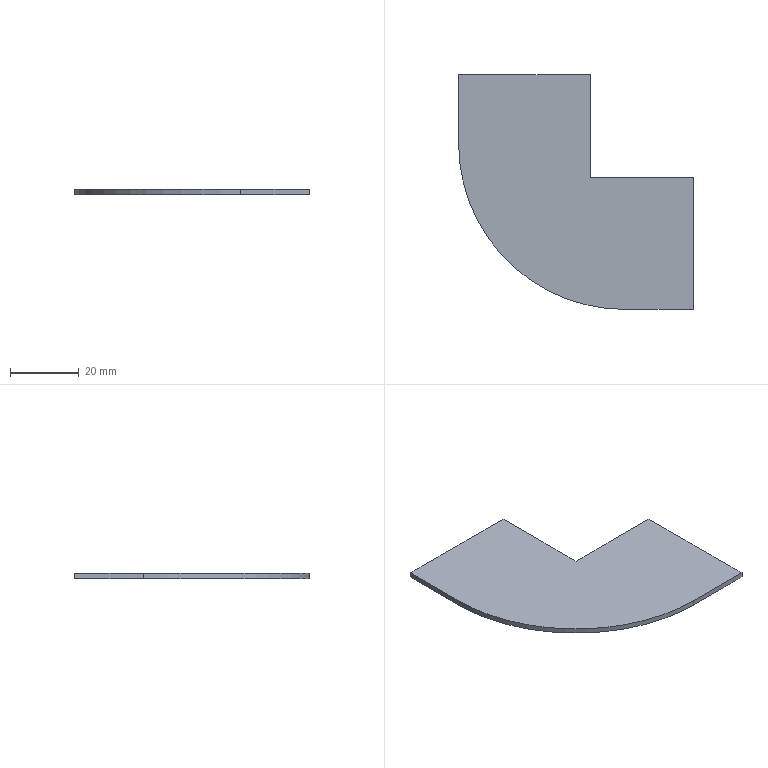Part | SolidWorks | features MirrorStock 1 | 1 solid | 9 faces | box 68.3 x 68.3 x 1.5 mm | volume 4896 mm3 | plane 8 | cylinder 1 | commonest cylinder face diameters 96.6 x1
STEP:
#1=CARTESIAN_POINT('',(9.455,94.386,0.));
#2=VERTEX_POINT('',#1);
#3=CARTESIAN_POINT('',(-28.845,94.386,0.));
#4=VERTEX_POINT('',#3);
#5=CARTESIAN_POINT('',(9.455,94.386,0.));
#6=DIRECTION('',(-1.,0.,0.));
#7=VECTOR('',#6,1000.);
#8=LINE('',#5,#7);
#9=EDGE_CURVE('',#2,#4,#8,.T.);
#10=ORIENTED_EDGE('',*,*,#9,.T.);
#11=CARTESIAN_POINT('',(-28.845,94.386,1.5));
#12=VERTEX_POINT('',#11);
#13=CARTESIAN_POINT('',(-28.845,94.386,1.5));
#14=DIRECTION('',(0.,0.,-1.));
#15=VECTOR('',#14,1000.);
#16=LINE('',#13,#15);
#17=EDGE_CURVE('',#12,#4,#16,.T.);
#18=ORIENTED_EDGE('',*,*,#17,.F.);
#19=CARTESIAN_POINT('',(9.455,94.386,1.5));
#20=VERTEX_POINT('',#19);
#21=CARTESIAN_POINT('',(9.455,94.386,1.5));
#22=DIRECTION('',(-1.,0.,0.));
#23=VECTOR('',#22,1000.);
#24=LINE('',#21,#23);
#25=EDGE_CURVE('',#20,#12,#24,.T.);
#26=ORIENTED_EDGE('',*,*,#25,.F.);
#27=CARTESIAN_POINT('',(9.455,94.386,1.5));
#28=DIRECTION('',(0.,0.,-1.));
#29=VECTOR('',#28,1000.);
#30=LINE('',#27,#29);
#31=EDGE_CURVE('',#20,#2,#30,.T.);
#32=ORIENTED_EDGE('',*,*,#31,.T.);
#33=EDGE_LOOP('',(#10,#18,#26,#32));
#34=FACE_OUTER_BOUND('',#33,.T.);
#35=CARTESIAN_POINT('',(9.455,94.386,1.5));
#36=DIRECTION('',(0.,1.,0.));
#37=DIRECTION('',(0.,0.,-1.));
#38=AXIS2_PLACEMENT_3D('',#35,#36,#37);
#39=PLANE('',#38);
#40=ADVANCED_FACE('',(#34),#39,.T.);
#41=CARTESIAN_POINT('',(9.455,64.386,0.));
#42=VERTEX_POINT('',#41);
#43=CARTESIAN_POINT('',(9.455,64.386,0.));
#44=DIRECTION('',(0.,1.,0.));
#45=VECTOR('',#44,1000.);
#46=LINE('',#43,#45);
#47=EDGE_CURVE('',#42,#2,#46,.T.);
#48=ORIENTED_EDGE('',*,*,#47,.T.);
#49=ORIENTED_EDGE('',*,*,#31,.F.);
#50=CARTESIAN_POINT('',(9.455,64.386,1.5));
#51=VERTEX_POINT('',#50);
#52=CARTESIAN_POINT('',(9.455,64.386,1.5));
#53=DIRECTION('',(0.,1.,0.));
#54=VECTOR('',#53,1000.);
#55=LINE('',#52,#54);
#56=EDGE_CURVE('',#51,#20,#55,.T.);
#57=ORIENTED_EDGE('',*,*,#56,.F.);
#58=CARTESIAN_POINT('',(9.455,64.386,1.5));
#59=DIRECTION('',(0.,0.,-1.));
#60=VECTOR('',#59,1000.);
#61=LINE('',#58,#60);
#62=EDGE_CURVE('',#51,#42,#61,.T.);
#63=ORIENTED_EDGE('',*,*,#62,.T.);
#64=EDGE_LOOP('',(#48,#49,#57,#63));
#65=FACE_OUTER_BOUND('',#64,.T.);
#66=CARTESIAN_POINT('',(9.455,64.386,1.5));
#67=DIRECTION('',(1.,0.,0.));
#68=DIRECTION('',(0.,0.,1.));
#69=AXIS2_PLACEMENT_3D('',#66,#67,#68);
#70=PLANE('',#69);
#71=ADVANCED_FACE('',(#65),#70,.T.);
#72=CARTESIAN_POINT('',(39.455,64.386,0.));
#73=VERTEX_POINT('',#72);
#74=CARTESIAN_POINT('',(39.455,64.386,0.));
#75=DIRECTION('',(-1.,0.,0.));
#76=VECTOR('',#75,1000.);
#77=LINE('',#74,#76);
#78=EDGE_CURVE('',#73,#42,#77,.T.);
#79=ORIENTED_EDGE('',*,*,#78,.T.);
#80=ORIENTED_EDGE('',*,*,#62,.F.);
#81=CARTESIAN_POINT('',(39.455,64.386,1.5));
#82=VERTEX_POINT('',#81);
#83=CARTESIAN_POINT('',(39.455,64.386,1.5));
#84=DIRECTION('',(-1.,0.,0.));
#85=VECTOR('',#84,1000.);
#86=LINE('',#83,#85);
#87=EDGE_CURVE('',#82,#51,#86,.T.);
#88=ORIENTED_EDGE('',*,*,#87,.F.);
#89=CARTESIAN_POINT('',(39.455,64.386,1.5));
#90=DIRECTION('',(0.,0.,-1.));
#91=VECTOR('',#90,1000.);
#92=LINE('',#89,#91);
#93=EDGE_CURVE('',#82,#73,#92,.T.);
#94=ORIENTED_EDGE('',*,*,#93,.T.);
#95=EDGE_LOOP('',(#79,#80,#88,#94));
#96=FACE_OUTER_BOUND('',#95,.T.);
#97=CARTESIAN_POINT('',(39.455,64.386,1.5));
#98=DIRECTION('',(0.,1.,0.));
#99=DIRECTION('',(-1.,0.,0.));
#100=AXIS2_PLACEMENT_3D('',#97,#98,#99);
#101=PLANE('',#100);
#102=ADVANCED_FACE('',(#96),#101,.T.);
#103=CARTESIAN_POINT('',(39.455,26.086,0.));
#104=VERTEX_POINT('',#103);
#105=CARTESIAN_POINT('',(39.455,26.086,0.));
#106=DIRECTION('',(0.,1.,0.));
#107=VECTOR('',#106,1000.);
#108=LINE('',#105,#107);
#109=EDGE_CURVE('',#104,#73,#108,.T.);
#110=ORIENTED_EDGE('',*,*,#109,.T.);
#111=ORIENTED_EDGE('',*,*,#93,.F.);
#112=CARTESIAN_POINT('',(39.455,26.086,1.5));
#113=VERTEX_POINT('',#112);
#114=CARTESIAN_POINT('',(39.455,26.086,1.5));
#115=DIRECTION('',(0.,1.,0.));
#116=VECTOR('',#115,1000.);
#117=LINE('',#114,#116);
#118=EDGE_CURVE('',#113,#82,#117,.T.);
#119=ORIENTED_EDGE('',*,*,#118,.F.);
#120=CARTESIAN_POINT('',(39.455,26.086,1.5));
#121=DIRECTION('',(0.,0.,-1.));
#122=VECTOR('',#121,1000.);
#123=LINE('',#120,#122);
#124=EDGE_CURVE('',#113,#104,#123,.T.);
#125=ORIENTED_EDGE('',*,*,#124,.T.);
#126=EDGE_LOOP('',(#110,#111,#119,#125));
#127=FACE_OUTER_BOUND('',#126,.T.);
#128=CARTESIAN_POINT('',(39.455,26.086,1.5));
#129=DIRECTION('',(1.,0.,0.));
#130=DIRECTION('',(0.,0.,1.));
#131=AXIS2_PLACEMENT_3D('',#128,#129,#130);
#132=PLANE('',#131);
#133=ADVANCED_FACE('',(#127),#132,.T.);
#134=CARTESIAN_POINT('',(19.455,26.086,0.));
#135=VERTEX_POINT('',#134);
#136=CARTESIAN_POINT('',(19.455,26.086,0.));
#137=DIRECTION('',(1.,0.,0.));
#138=VECTOR('',#137,1000.);
#139=LINE('',#136,#138);
#140=EDGE_CURVE('',#135,#104,#139,.T.);
#141=ORIENTED_EDGE('',*,*,#140,.T.);
#142=ORIENTED_EDGE('',*,*,#124,.F.);
#143=CARTESIAN_POINT('',(19.455,26.086,1.5));
#144=VERTEX_POINT('',#143);
#145=CARTESIAN_POINT('',(19.455,26.086,1.5));
#146=DIRECTION('',(1.,0.,0.));
#147=VECTOR('',#146,1000.);
#148=LINE('',#145,#147);
#149=EDGE_CURVE('',#144,#113,#148,.T.);
#150=ORIENTED_EDGE('',*,*,#149,.F.);
#151=CARTESIAN_POINT('',(19.455,26.086,1.5));
#152=DIRECTION('',(0.,0.,-1.));
#153=VECTOR('',#152,1000.);
#154=LINE('',#151,#153);
#155=EDGE_CURVE('',#144,#135,#154,.T.);
#156=ORIENTED_EDGE('',*,*,#155,.T.);
#157=EDGE_LOOP('',(#141,#142,#150,#156));
#158=FACE_OUTER_BOUND('',#157,.T.);
#159=CARTESIAN_POINT('',(19.455,26.086,1.5));
#160=DIRECTION('',(0.,-1.,0.));
#161=DIRECTION('',(0.,0.,1.));
#162=AXIS2_PLACEMENT_3D('',#159,#160,#161);
#163=PLANE('',#162);
#164=ADVANCED_FACE('',(#158),#163,.T.);
#165=CARTESIAN_POINT('',(-28.845,74.386,0.));
#166=VERTEX_POINT('',#165);
#167=CARTESIAN_POINT('',(19.455,74.386,0.));
#168=DIRECTION('',(0.,0.,1.));
#169=DIRECTION('',(-1.,0.,0.));
#170=AXIS2_PLACEMENT_3D('',#167,#168,#169);
#171=CIRCLE('',#170,48.3);
#172=EDGE_CURVE('',#166,#135,#171,.T.);
#173=ORIENTED_EDGE('',*,*,#172,.T.);
#174=ORIENTED_EDGE('',*,*,#155,.F.);
#175=CARTESIAN_POINT('',(-28.845,74.386,1.5));
#176=VERTEX_POINT('',#175);
#177=CARTESIAN_POINT('',(19.455,74.386,1.5));
#178=DIRECTION('',(0.,0.,1.));
#179=DIRECTION('',(-1.,0.,0.));
#180=AXIS2_PLACEMENT_3D('',#177,#178,#179);
#181=CIRCLE('',#180,48.3);
#182=EDGE_CURVE('',#176,#144,#181,.T.);
#183=ORIENTED_EDGE('',*,*,#182,.F.);
#184=CARTESIAN_POINT('',(-28.845,74.386,1.5));
#185=DIRECTION('',(0.,0.,-1.));
#186=VECTOR('',#185,1000.);
#187=LINE('',#184,#186);
#188=EDGE_CURVE('',#176,#166,#187,.T.);
#189=ORIENTED_EDGE('',*,*,#188,.T.);
#190=EDGE_LOOP('',(#173,#174,#183,#189));
#191=FACE_OUTER_BOUND('',#190,.T.);
#192=CARTESIAN_POINT('',(19.455,74.386,1.5));
#193=DIRECTION('',(0.,0.,-1.));
#194=DIRECTION('',(1.,0.,0.));
#195=AXIS2_PLACEMENT_3D('',#192,#193,#194);
#196=CYLINDRICAL_SURFACE('',#195,48.3);
#197=ADVANCED_FACE('',(#191),#196,.T.);
#198=CARTESIAN_POINT('',(-28.845,94.386,0.));
#199=DIRECTION('',(0.,-1.,0.));
#200=VECTOR('',#199,1000.);
#201=LINE('',#198,#200);
#202=EDGE_CURVE('',#4,#166,#201,.T.);
#203=ORIENTED_EDGE('',*,*,#202,.T.);
#204=ORIENTED_EDGE('',*,*,#188,.F.);
#205=CARTESIAN_POINT('',(-28.845,94.386,1.5));
#206=DIRECTION('',(0.,-1.,0.));
#207=VECTOR('',#206,1000.);
#208=LINE('',#205,#207);
#209=EDGE_CURVE('',#12,#176,#208,.T.);
#210=ORIENTED_EDGE('',*,*,#209,.F.);
#211=ORIENTED_EDGE('',*,*,#17,.T.);
#212=EDGE_LOOP('',(#203,#204,#210,#211));
#213=FACE_OUTER_BOUND('',#212,.T.);
#214=CARTESIAN_POINT('',(-28.845,94.386,1.5));
#215=DIRECTION('',(-1.,0.,0.));
#216=DIRECTION('',(0.,-1.,0.));
#217=AXIS2_PLACEMENT_3D('',#214,#215,#216);
#218=PLANE('',#217);
#219=ADVANCED_FACE('',(#213),#218,.T.);
#220=ORIENTED_EDGE('',*,*,#25,.T.);
#221=ORIENTED_EDGE('',*,*,#209,.T.);
#222=ORIENTED_EDGE('',*,*,#182,.T.);
#223=ORIENTED_EDGE('',*,*,#149,.T.);
#224=ORIENTED_EDGE('',*,*,#118,.T.);
#225=ORIENTED_EDGE('',*,*,#87,.T.);
#226=ORIENTED_EDGE('',*,*,#56,.T.);
#227=EDGE_LOOP('',(#220,#221,#222,#223,#224,#225,#226));
#228=FACE_OUTER_BOUND('',#227,.T.);
#229=CARTESIAN_POINT('',(19.455,74.386,1.5));
#230=DIRECTION('',(0.,0.,1.));
#231=DIRECTION('',(-1.,0.,0.));
#232=AXIS2_PLACEMENT_3D('',#229,#230,#231);
#233=PLANE('',#232);
#234=ADVANCED_FACE('',(#228),#233,.T.);
#235=ORIENTED_EDGE('',*,*,#9,.F.);
#236=ORIENTED_EDGE('',*,*,#47,.F.);
#237=ORIENTED_EDGE('',*,*,#78,.F.);
#238=ORIENTED_EDGE('',*,*,#109,.F.);
#239=ORIENTED_EDGE('',*,*,#140,.F.);
#240=ORIENTED_EDGE('',*,*,#172,.F.);
#241=ORIENTED_EDGE('',*,*,#202,.F.);
#242=EDGE_LOOP('',(#235,#236,#237,#238,#239,#240,#241));
#243=FACE_OUTER_BOUND('',#242,.T.);
#244=CARTESIAN_POINT('',(19.455,74.386,0.));
#245=DIRECTION('',(0.,0.,1.));
#246=DIRECTION('',(-1.,0.,0.));
#247=AXIS2_PLACEMENT_3D('',#244,#245,#246);
#248=PLANE('',#247);
#249=ADVANCED_FACE('',(#243),#248,.F.);
#250=CLOSED_SHELL('',(#40,#71,#102,#133,#164,#197,#219,#234,#249));
#251=MANIFOLD_SOLID_BREP('',#250);
#252=CARTESIAN_POINT('',(0.,0.,0.));
#253=DIRECTION('',(0.,0.,1.));
#254=DIRECTION('',(1.,0.,0.));
#255=AXIS2_PLACEMENT_3D('',#252,#253,#254);
#256=(LENGTH_UNIT()NAMED_UNIT(*)SI_UNIT(.MILLI.,.METRE.));
#257=UNCERTAINTY_MEASURE_WITH_UNIT(LENGTH_MEASURE(0.00001),#256,'','');
#258=(NAMED_UNIT(*)PLANE_ANGLE_UNIT()SI_UNIT($,.RADIAN.));
#259=(NAMED_UNIT(*)SI_UNIT($,.STERADIAN.)SOLID_ANGLE_UNIT());
#260=(GEOMETRIC_REPRESENTATION_CONTEXT(3)GLOBAL_UNCERTAINTY_ASSIGNED_CONTEXT((#257))GLOBAL_UNIT_ASSIGNED_CONTEXT((#256,#258,#259))REPRESENTATION_CONTEXT('',''));
#261=ADVANCED_BREP_SHAPE_REPRESENTATION('',(#251,#255),#260);